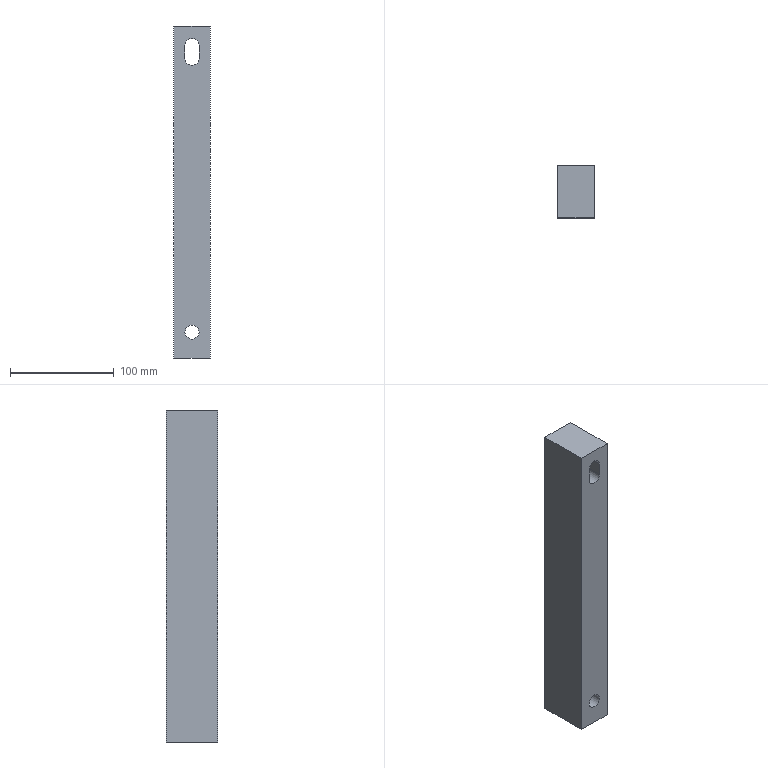Part | NX | features solid 2 | 1 solid | 11 faces | box 35 x 50 x 320 mm | volume 537249 mm3 | plane 8 | cylinder 3 | commonest cylinder face diameters 13.5 x3
STEP:
#1=CARTESIAN_POINT('',(-933.25,-373.,136.25));
#2=VERTEX_POINT('',#1);
#3=CARTESIAN_POINT('',(-946.75,-373.,136.25));
#4=VERTEX_POINT('',#3);
#5=CARTESIAN_POINT('',(-940.,-373.,136.25));
#6=DIRECTION('',(0.,-1.,0.));
#7=DIRECTION('',(1.,0.,0.));
#8=AXIS2_PLACEMENT_3D('',#5,#6,#7);
#9=CIRCLE('',#8,6.75);
#10=EDGE_CURVE('',#2,#4,#9,.T.);
#11=ORIENTED_EDGE('',*,*,#10,.T.);
#12=CARTESIAN_POINT('',(-946.75,-323.,136.25));
#13=VERTEX_POINT('',#12);
#14=CARTESIAN_POINT('',(-946.75,-323.,136.25));
#15=DIRECTION('',(0.,-1.,0.));
#16=VECTOR('',#15,1000.);
#17=LINE('',#14,#16);
#18=EDGE_CURVE('',#13,#4,#17,.T.);
#19=ORIENTED_EDGE('',*,*,#18,.F.);
#20=CARTESIAN_POINT('',(-933.25,-323.,136.25));
#21=VERTEX_POINT('',#20);
#22=CARTESIAN_POINT('',(-940.,-323.,136.25));
#23=DIRECTION('',(0.,-1.,0.));
#24=DIRECTION('',(1.,0.,0.));
#25=AXIS2_PLACEMENT_3D('',#22,#23,#24);
#26=CIRCLE('',#25,6.75);
#27=EDGE_CURVE('',#21,#13,#26,.T.);
#28=ORIENTED_EDGE('',*,*,#27,.F.);
#29=CARTESIAN_POINT('',(-933.25,-323.,136.25));
#30=DIRECTION('',(0.,-1.,0.));
#31=VECTOR('',#30,1000.);
#32=LINE('',#29,#31);
#33=EDGE_CURVE('',#21,#2,#32,.T.);
#34=ORIENTED_EDGE('',*,*,#33,.T.);
#35=EDGE_LOOP('',(#11,#19,#28,#34));
#36=FACE_BOUND('',#35,.T.);
#37=CARTESIAN_POINT('',(-940.,-323.,136.25));
#38=DIRECTION('',(0.,-1.,0.));
#39=DIRECTION('',(0.,0.,-1.));
#40=AXIS2_PLACEMENT_3D('',#37,#38,#39);
#41=CYLINDRICAL_SURFACE('',#40,6.75);
#42=ADVANCED_FACE('',(#36),#41,.F.);
#43=CARTESIAN_POINT('',(-933.25,-373.,123.75));
#44=VERTEX_POINT('',#43);
#45=CARTESIAN_POINT('',(-933.25,-373.,136.25));
#46=DIRECTION('',(0.,0.,-1.));
#47=VECTOR('',#46,1000.);
#48=LINE('',#45,#47);
#49=EDGE_CURVE('',#2,#44,#48,.T.);
#50=ORIENTED_EDGE('',*,*,#49,.F.);
#51=ORIENTED_EDGE('',*,*,#33,.F.);
#52=CARTESIAN_POINT('',(-933.25,-323.,123.75));
#53=VERTEX_POINT('',#52);
#54=CARTESIAN_POINT('',(-933.25,-323.,136.25));
#55=DIRECTION('',(0.,0.,-1.));
#56=VECTOR('',#55,1000.);
#57=LINE('',#54,#56);
#58=EDGE_CURVE('',#21,#53,#57,.T.);
#59=ORIENTED_EDGE('',*,*,#58,.T.);
#60=CARTESIAN_POINT('',(-933.25,-323.,123.75));
#61=DIRECTION('',(0.,-1.,0.));
#62=VECTOR('',#61,1000.);
#63=LINE('',#60,#62);
#64=EDGE_CURVE('',#53,#44,#63,.T.);
#65=ORIENTED_EDGE('',*,*,#64,.T.);
#66=EDGE_LOOP('',(#50,#51,#59,#65));
#67=FACE_BOUND('',#66,.T.);
#68=CARTESIAN_POINT('',(-933.25,-323.,136.25));
#69=DIRECTION('',(-1.,0.,0.));
#70=DIRECTION('',(0.,0.,1.));
#71=AXIS2_PLACEMENT_3D('',#68,#69,#70);
#72=PLANE('',#71);
#73=ADVANCED_FACE('',(#67),#72,.T.);
#74=CARTESIAN_POINT('',(-946.75,-373.,123.75));
#75=VERTEX_POINT('',#74);
#76=CARTESIAN_POINT('',(-940.,-373.,123.75));
#77=DIRECTION('',(0.,-1.,0.));
#78=DIRECTION('',(1.,0.,0.));
#79=AXIS2_PLACEMENT_3D('',#76,#77,#78);
#80=CIRCLE('',#79,6.75);
#81=EDGE_CURVE('',#75,#44,#80,.T.);
#82=ORIENTED_EDGE('',*,*,#81,.T.);
#83=ORIENTED_EDGE('',*,*,#64,.F.);
#84=CARTESIAN_POINT('',(-946.75,-323.,123.75));
#85=VERTEX_POINT('',#84);
#86=CARTESIAN_POINT('',(-940.,-323.,123.75));
#87=DIRECTION('',(0.,-1.,0.));
#88=DIRECTION('',(1.,0.,0.));
#89=AXIS2_PLACEMENT_3D('',#86,#87,#88);
#90=CIRCLE('',#89,6.75);
#91=EDGE_CURVE('',#85,#53,#90,.T.);
#92=ORIENTED_EDGE('',*,*,#91,.F.);
#93=CARTESIAN_POINT('',(-946.75,-323.,123.75));
#94=DIRECTION('',(0.,-1.,0.));
#95=VECTOR('',#94,1000.);
#96=LINE('',#93,#95);
#97=EDGE_CURVE('',#85,#75,#96,.T.);
#98=ORIENTED_EDGE('',*,*,#97,.T.);
#99=EDGE_LOOP('',(#82,#83,#92,#98));
#100=FACE_BOUND('',#99,.T.);
#101=CARTESIAN_POINT('',(-940.,-323.,123.75));
#102=DIRECTION('',(0.,-1.,0.));
#103=DIRECTION('',(0.,0.,-1.));
#104=AXIS2_PLACEMENT_3D('',#101,#102,#103);
#105=CYLINDRICAL_SURFACE('',#104,6.75);
#106=ADVANCED_FACE('',(#100),#105,.F.);
#107=CARTESIAN_POINT('',(-957.5,-373.,155.));
#108=VERTEX_POINT('',#107);
#109=CARTESIAN_POINT('',(-957.5,-373.,-165.));
#110=VERTEX_POINT('',#109);
#111=CARTESIAN_POINT('',(-957.5,-373.,215.));
#112=DIRECTION('',(0.,0.,-1.));
#113=VECTOR('',#112,1000.);
#114=LINE('',#111,#113);
#115=EDGE_CURVE('',#108,#110,#114,.T.);
#116=ORIENTED_EDGE('',*,*,#115,.F.);
#117=CARTESIAN_POINT('',(-957.5,-323.,155.));
#118=VERTEX_POINT('',#117);
#119=CARTESIAN_POINT('',(-957.5,-323.,155.));
#120=DIRECTION('',(0.,-1.,0.));
#121=VECTOR('',#120,1000.);
#122=LINE('',#119,#121);
#123=EDGE_CURVE('',#118,#108,#122,.T.);
#124=ORIENTED_EDGE('',*,*,#123,.F.);
#125=CARTESIAN_POINT('',(-957.5,-323.,-165.));
#126=VERTEX_POINT('',#125);
#127=CARTESIAN_POINT('',(-957.5,-323.,215.));
#128=DIRECTION('',(0.,0.,-1.));
#129=VECTOR('',#128,1000.);
#130=LINE('',#127,#129);
#131=EDGE_CURVE('',#118,#126,#130,.T.);
#132=ORIENTED_EDGE('',*,*,#131,.T.);
#133=CARTESIAN_POINT('',(-957.5,-323.,-165.));
#134=DIRECTION('',(0.,-1.,0.));
#135=VECTOR('',#134,1000.);
#136=LINE('',#133,#135);
#137=EDGE_CURVE('',#126,#110,#136,.T.);
#138=ORIENTED_EDGE('',*,*,#137,.T.);
#139=EDGE_LOOP('',(#116,#124,#132,#138));
#140=FACE_BOUND('',#139,.T.);
#141=CARTESIAN_POINT('',(-957.5,-323.,215.));
#142=DIRECTION('',(-1.,0.,0.));
#143=DIRECTION('',(0.,0.,1.));
#144=AXIS2_PLACEMENT_3D('',#141,#142,#143);
#145=PLANE('',#144);
#146=ADVANCED_FACE('',(#140),#145,.T.);
#147=CARTESIAN_POINT('',(-922.5,-373.,-165.));
#148=VERTEX_POINT('',#147);
#149=CARTESIAN_POINT('',(-957.5,-373.,-165.));
#150=DIRECTION('',(1.,0.,0.));
#151=VECTOR('',#150,1000.);
#152=LINE('',#149,#151);
#153=EDGE_CURVE('',#110,#148,#152,.T.);
#154=ORIENTED_EDGE('',*,*,#153,.F.);
#155=ORIENTED_EDGE('',*,*,#137,.F.);
#156=CARTESIAN_POINT('',(-922.5,-323.,-165.));
#157=VERTEX_POINT('',#156);
#158=CARTESIAN_POINT('',(-957.5,-323.,-165.));
#159=DIRECTION('',(1.,0.,0.));
#160=VECTOR('',#159,1000.);
#161=LINE('',#158,#160);
#162=EDGE_CURVE('',#126,#157,#161,.T.);
#163=ORIENTED_EDGE('',*,*,#162,.T.);
#164=CARTESIAN_POINT('',(-922.5,-323.,-165.));
#165=DIRECTION('',(0.,-1.,0.));
#166=VECTOR('',#165,1000.);
#167=LINE('',#164,#166);
#168=EDGE_CURVE('',#157,#148,#167,.T.);
#169=ORIENTED_EDGE('',*,*,#168,.T.);
#170=EDGE_LOOP('',(#154,#155,#163,#169));
#171=FACE_BOUND('',#170,.T.);
#172=CARTESIAN_POINT('',(-957.5,-323.,-165.));
#173=DIRECTION('',(0.,0.,-1.));
#174=DIRECTION('',(-1.,0.,0.));
#175=AXIS2_PLACEMENT_3D('',#172,#173,#174);
#176=PLANE('',#175);
#177=ADVANCED_FACE('',(#171),#176,.T.);
#178=CARTESIAN_POINT('',(-922.5,-373.,155.));
#179=VERTEX_POINT('',#178);
#180=CARTESIAN_POINT('',(-922.5,-373.,-85.));
#181=DIRECTION('',(0.,0.,1.));
#182=VECTOR('',#181,1000.);
#183=LINE('',#180,#182);
#184=EDGE_CURVE('',#148,#179,#183,.T.);
#185=ORIENTED_EDGE('',*,*,#184,.F.);
#186=ORIENTED_EDGE('',*,*,#168,.F.);
#187=CARTESIAN_POINT('',(-922.5,-323.,155.));
#188=VERTEX_POINT('',#187);
#189=CARTESIAN_POINT('',(-922.5,-323.,-85.));
#190=DIRECTION('',(0.,0.,1.));
#191=VECTOR('',#190,1000.);
#192=LINE('',#189,#191);
#193=EDGE_CURVE('',#157,#188,#192,.T.);
#194=ORIENTED_EDGE('',*,*,#193,.T.);
#195=CARTESIAN_POINT('',(-922.5,-323.,155.));
#196=DIRECTION('',(0.,-1.,0.));
#197=VECTOR('',#196,1000.);
#198=LINE('',#195,#197);
#199=EDGE_CURVE('',#188,#179,#198,.T.);
#200=ORIENTED_EDGE('',*,*,#199,.T.);
#201=EDGE_LOOP('',(#185,#186,#194,#200));
#202=FACE_BOUND('',#201,.T.);
#203=CARTESIAN_POINT('',(-922.5,-323.,-85.));
#204=DIRECTION('',(1.,0.,0.));
#205=DIRECTION('',(0.,0.,-1.));
#206=AXIS2_PLACEMENT_3D('',#203,#204,#205);
#207=PLANE('',#206);
#208=ADVANCED_FACE('',(#202),#207,.T.);
#209=CARTESIAN_POINT('',(-933.25,-323.,-140.));
#210=VERTEX_POINT('',#209);
#211=CARTESIAN_POINT('',(-940.,-323.,-140.));
#212=DIRECTION('',(0.,-1.,0.));
#213=DIRECTION('',(1.,0.,0.));
#214=AXIS2_PLACEMENT_3D('',#211,#212,#213);
#215=CIRCLE('',#214,6.75);
#216=EDGE_CURVE('',#210,#210,#215,.T.);
#217=ORIENTED_EDGE('',*,*,#216,.F.);
#218=EDGE_LOOP('',(#217));
#219=FACE_BOUND('',#218,.T.);
#220=CARTESIAN_POINT('',(-933.25,-373.,-140.));
#221=VERTEX_POINT('',#220);
#222=CARTESIAN_POINT('',(-940.,-373.,-140.));
#223=DIRECTION('',(0.,-1.,0.));
#224=DIRECTION('',(1.,0.,0.));
#225=AXIS2_PLACEMENT_3D('',#222,#223,#224);
#226=CIRCLE('',#225,6.75);
#227=EDGE_CURVE('',#221,#221,#226,.T.);
#228=ORIENTED_EDGE('',*,*,#227,.T.);
#229=EDGE_LOOP('',(#228));
#230=FACE_BOUND('',#229,.T.);
#231=CARTESIAN_POINT('',(-940.,-323.,-140.));
#232=DIRECTION('',(0.,-1.,0.));
#233=DIRECTION('',(0.,0.,-1.));
#234=AXIS2_PLACEMENT_3D('',#231,#232,#233);
#235=CYLINDRICAL_SURFACE('',#234,6.75);
#236=ADVANCED_FACE('',(#219,#230),#235,.F.);
#237=CARTESIAN_POINT('',(-922.5,-373.,155.));
#238=DIRECTION('',(-1.,0.,0.));
#239=VECTOR('',#238,1000.);
#240=LINE('',#237,#239);
#241=EDGE_CURVE('',#179,#108,#240,.T.);
#242=ORIENTED_EDGE('',*,*,#241,.F.);
#243=ORIENTED_EDGE('',*,*,#199,.F.);
#244=CARTESIAN_POINT('',(-922.5,-323.,155.));
#245=DIRECTION('',(-1.,0.,0.));
#246=VECTOR('',#245,1000.);
#247=LINE('',#244,#246);
#248=EDGE_CURVE('',#188,#118,#247,.T.);
#249=ORIENTED_EDGE('',*,*,#248,.T.);
#250=ORIENTED_EDGE('',*,*,#123,.T.);
#251=EDGE_LOOP('',(#242,#243,#249,#250));
#252=FACE_BOUND('',#251,.T.);
#253=CARTESIAN_POINT('',(-922.5,-323.,155.));
#254=DIRECTION('',(0.,0.,1.));
#255=DIRECTION('',(1.,0.,0.));
#256=AXIS2_PLACEMENT_3D('',#253,#254,#255);
#257=PLANE('',#256);
#258=ADVANCED_FACE('',(#252),#257,.T.);
#259=CARTESIAN_POINT('',(-946.75,-373.,123.75));
#260=DIRECTION('',(0.,0.,1.));
#261=VECTOR('',#260,1000.);
#262=LINE('',#259,#261);
#263=EDGE_CURVE('',#75,#4,#262,.T.);
#264=ORIENTED_EDGE('',*,*,#263,.F.);
#265=ORIENTED_EDGE('',*,*,#97,.F.);
#266=CARTESIAN_POINT('',(-946.75,-323.,123.75));
#267=DIRECTION('',(0.,0.,1.));
#268=VECTOR('',#267,1000.);
#269=LINE('',#266,#268);
#270=EDGE_CURVE('',#85,#13,#269,.T.);
#271=ORIENTED_EDGE('',*,*,#270,.T.);
#272=ORIENTED_EDGE('',*,*,#18,.T.);
#273=EDGE_LOOP('',(#264,#265,#271,#272));
#274=FACE_BOUND('',#273,.T.);
#275=CARTESIAN_POINT('',(-946.75,-323.,123.75));
#276=DIRECTION('',(1.,0.,0.));
#277=DIRECTION('',(0.,0.,-1.));
#278=AXIS2_PLACEMENT_3D('',#275,#276,#277);
#279=PLANE('',#278);
#280=ADVANCED_FACE('',(#274),#279,.T.);
#281=ORIENTED_EDGE('',*,*,#131,.F.);
#282=ORIENTED_EDGE('',*,*,#248,.F.);
#283=ORIENTED_EDGE('',*,*,#193,.F.);
#284=ORIENTED_EDGE('',*,*,#162,.F.);
#285=EDGE_LOOP('',(#281,#282,#283,#284));
#286=FACE_BOUND('',#285,.T.);
#287=ORIENTED_EDGE('',*,*,#216,.T.);
#288=EDGE_LOOP('',(#287));
#289=FACE_BOUND('',#288,.T.);
#290=ORIENTED_EDGE('',*,*,#27,.T.);
#291=ORIENTED_EDGE('',*,*,#270,.F.);
#292=ORIENTED_EDGE('',*,*,#91,.T.);
#293=ORIENTED_EDGE('',*,*,#58,.F.);
#294=EDGE_LOOP('',(#290,#291,#292,#293));
#295=FACE_BOUND('',#294,.T.);
#296=CARTESIAN_POINT('',(-922.5,-323.,215.));
#297=DIRECTION('',(0.,1.,0.));
#298=DIRECTION('',(1.,0.,0.));
#299=AXIS2_PLACEMENT_3D('',#296,#297,#298);
#300=PLANE('',#299);
#301=ADVANCED_FACE('',(#286,#289,#295),#300,.T.);
#302=ORIENTED_EDGE('',*,*,#115,.T.);
#303=ORIENTED_EDGE('',*,*,#153,.T.);
#304=ORIENTED_EDGE('',*,*,#184,.T.);
#305=ORIENTED_EDGE('',*,*,#241,.T.);
#306=EDGE_LOOP('',(#302,#303,#304,#305));
#307=FACE_BOUND('',#306,.T.);
#308=ORIENTED_EDGE('',*,*,#227,.F.);
#309=EDGE_LOOP('',(#308));
#310=FACE_BOUND('',#309,.T.);
#311=ORIENTED_EDGE('',*,*,#10,.F.);
#312=ORIENTED_EDGE('',*,*,#49,.T.);
#313=ORIENTED_EDGE('',*,*,#81,.F.);
#314=ORIENTED_EDGE('',*,*,#263,.T.);
#315=EDGE_LOOP('',(#311,#312,#313,#314));
#316=FACE_BOUND('',#315,.T.);
#317=CARTESIAN_POINT('',(-922.5,-373.,215.));
#318=DIRECTION('',(0.,1.,0.));
#319=DIRECTION('',(1.,0.,0.));
#320=AXIS2_PLACEMENT_3D('',#317,#318,#319);
#321=PLANE('',#320);
#322=ADVANCED_FACE('',(#307,#310,#316),#321,.F.);
#323=CLOSED_SHELL('',(#42,#73,#106,#146,#177,#208,#236,#258,#280,#301,#322));
#324=MANIFOLD_SOLID_BREP('',#323);
#325=(LENGTH_UNIT()NAMED_UNIT(*)SI_UNIT(.MILLI.,.METRE.));
#326=UNCERTAINTY_MEASURE_WITH_UNIT(LENGTH_MEASURE(0.00001),#325,'','');
#327=(NAMED_UNIT(*)PLANE_ANGLE_UNIT()SI_UNIT($,.RADIAN.));
#328=(NAMED_UNIT(*)SI_UNIT($,.STERADIAN.)SOLID_ANGLE_UNIT());
#329=(GEOMETRIC_REPRESENTATION_CONTEXT(3)GLOBAL_UNCERTAINTY_ASSIGNED_CONTEXT((#326))GLOBAL_UNIT_ASSIGNED_CONTEXT((#325,#327,#328))REPRESENTATION_CONTEXT('',''));
#330=ADVANCED_BREP_SHAPE_REPRESENTATION('',(#324),#329);